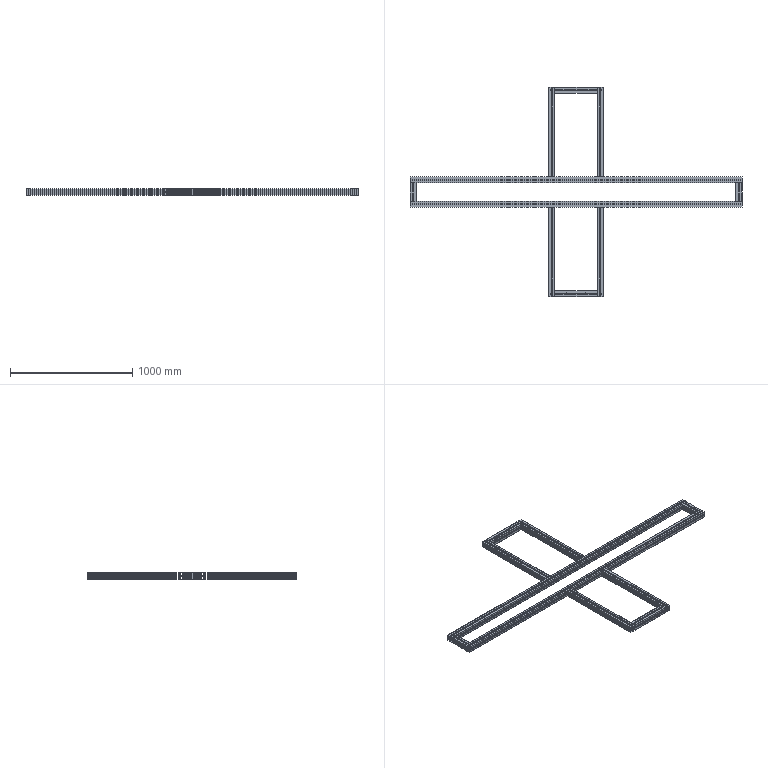Part | SolidWorks | features WeldCornerFeat 6, WeldMemberFeat 3, 3DProfileFeature 1, HoleWzd 1, WeldmentFeature 1 | 10 solids | 1136 faces | box 2720 x 1720 x 50 mm | volume 8199509 mm3 | plane 892 | cylinder 244 | commonest cylinder face diameters 14 x72 2.2 x60 9 x52 1 x40 15 x20